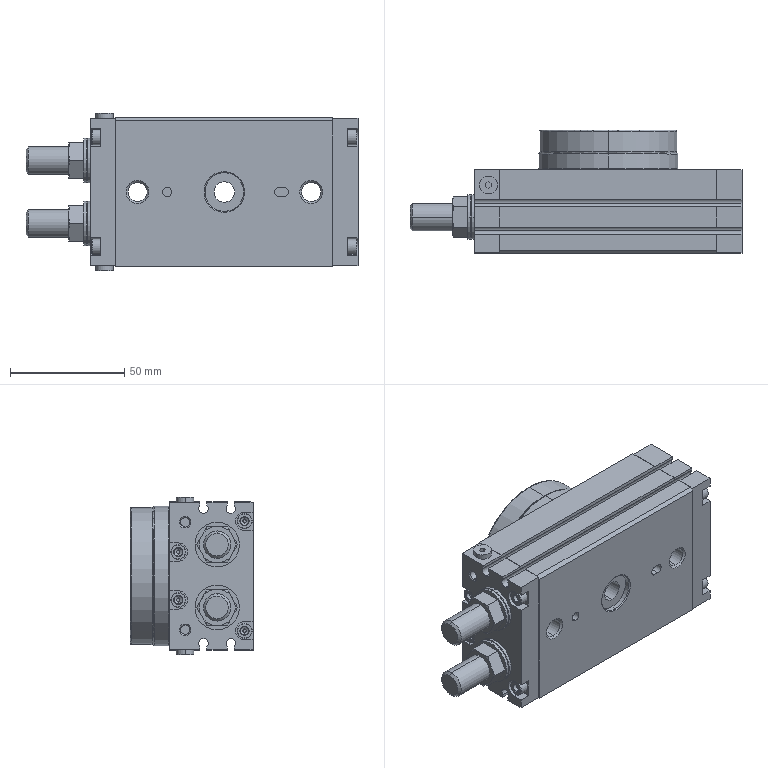Part | SolidWorks | 1 solid | 490 faces | box 145.3 x 54 x 69 mm | volume 311465 mm3 | plane 172 | cylinder 162 | cone 134 | spline 22 | commonest cylinder face diameters 6.66 x28 4.917 x24 3.5 x16 2.572 x12 4 x12 6.16 x12